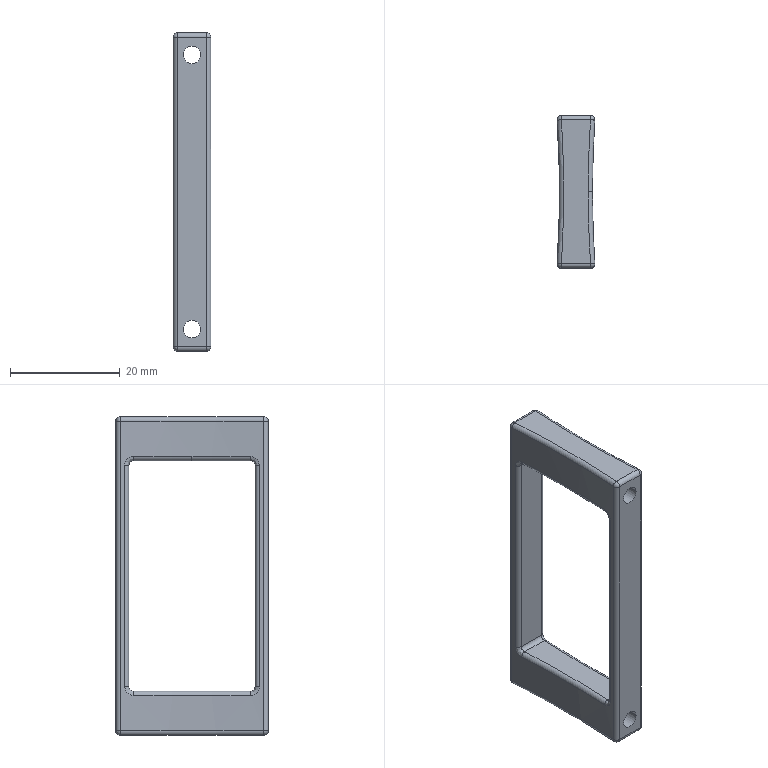Part | SolidWorks | features ICE 2, Extrusion 1, Fillet 1 | 1 solid | 65 faces | box 6.889 x 27.8 x 58 mm | volume 3675 mm3 | cylinder 25 | sphere 12 | torus 12 | plane 8 | spline 8 | commonest cylinder face diameters 1.6 x18 3.2 x4 400.965 x3